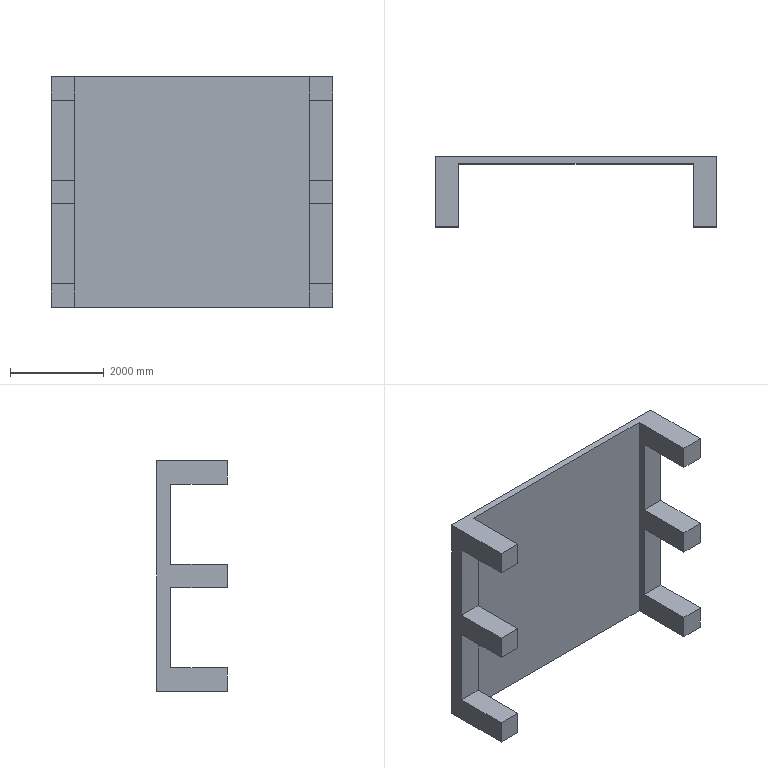Part | SolidWorks | features Extrusion 1, ICE 1 | 1 solid | 26 faces | box 6000 x 1500 x 4914 mm | volume 6959700000 mm3 | plane 26
STEP:
#1=CARTESIAN_POINT('',(2500.,-1500.,-65.));
#2=VERTEX_POINT('',#1);
#3=CARTESIAN_POINT('',(3000.,-1500.,-65.));
#4=VERTEX_POINT('',#3);
#5=CARTESIAN_POINT('',(-3000.,-1500.,-65.));
#6=DIRECTION('',(1.,0.,0.));
#7=VECTOR('',#6,1000.);
#8=LINE('',#5,#7);
#9=EDGE_CURVE('',#2,#4,#8,.T.);
#10=ORIENTED_EDGE('',*,*,#9,.T.);
#11=CARTESIAN_POINT('',(3000.,-1500.,435.));
#12=VERTEX_POINT('',#11);
#13=CARTESIAN_POINT('',(3000.,-1500.,-4479.));
#14=DIRECTION('',(0.,0.,1.));
#15=VECTOR('',#14,1000.);
#16=LINE('',#13,#15);
#17=EDGE_CURVE('',#4,#12,#16,.T.);
#18=ORIENTED_EDGE('',*,*,#17,.T.);
#19=CARTESIAN_POINT('',(2500.,-1500.,435.));
#20=VERTEX_POINT('',#19);
#21=CARTESIAN_POINT('',(3000.,-1500.,435.));
#22=DIRECTION('',(1.,0.,0.));
#23=VECTOR('',#22,1000.);
#24=LINE('',#21,#23);
#25=EDGE_CURVE('',#20,#12,#24,.T.);
#26=ORIENTED_EDGE('',*,*,#25,.F.);
#27=CARTESIAN_POINT('',(2500.,-1500.,-4479.));
#28=DIRECTION('',(0.,0.,1.));
#29=VECTOR('',#28,1000.);
#30=LINE('',#27,#29);
#31=EDGE_CURVE('',#2,#20,#30,.T.);
#32=ORIENTED_EDGE('',*,*,#31,.F.);
#33=EDGE_LOOP('',(#10,#18,#26,#32));
#34=FACE_OUTER_BOUND('',#33,.T.);
#35=CARTESIAN_POINT('',(3000.,-1500.,-4479.));
#36=DIRECTION('',(0.,-1.,0.));
#37=DIRECTION('',(1.,0.,0.));
#38=AXIS2_PLACEMENT_3D('',#35,#36,#37);
#39=PLANE('',#38);
#40=ADVANCED_FACE('',(#34),#39,.T.);
#41=CARTESIAN_POINT('',(2500.,-1500.,-1772.));
#42=VERTEX_POINT('',#41);
#43=CARTESIAN_POINT('',(3000.,-1500.,-1772.));
#44=VERTEX_POINT('',#43);
#45=CARTESIAN_POINT('',(-3000.,-1500.,-1772.));
#46=DIRECTION('',(1.,0.,0.));
#47=VECTOR('',#46,1000.);
#48=LINE('',#45,#47);
#49=EDGE_CURVE('',#42,#44,#48,.T.);
#50=ORIENTED_EDGE('',*,*,#49,.F.);
#51=CARTESIAN_POINT('',(2500.,-1500.,-2272.));
#52=VERTEX_POINT('',#51);
#53=CARTESIAN_POINT('',(2500.,-1500.,-4479.));
#54=DIRECTION('',(0.,0.,1.));
#55=VECTOR('',#54,1000.);
#56=LINE('',#53,#55);
#57=EDGE_CURVE('',#52,#42,#56,.T.);
#58=ORIENTED_EDGE('',*,*,#57,.F.);
#59=CARTESIAN_POINT('',(3000.,-1500.,-2272.));
#60=VERTEX_POINT('',#59);
#61=CARTESIAN_POINT('',(-3000.,-1500.,-2272.));
#62=DIRECTION('',(1.,0.,0.));
#63=VECTOR('',#62,1000.);
#64=LINE('',#61,#63);
#65=EDGE_CURVE('',#52,#60,#64,.T.);
#66=ORIENTED_EDGE('',*,*,#65,.T.);
#67=CARTESIAN_POINT('',(3000.,-1500.,-4479.));
#68=DIRECTION('',(0.,0.,1.));
#69=VECTOR('',#68,1000.);
#70=LINE('',#67,#69);
#71=EDGE_CURVE('',#60,#44,#70,.T.);
#72=ORIENTED_EDGE('',*,*,#71,.T.);
#73=EDGE_LOOP('',(#50,#58,#66,#72));
#74=FACE_OUTER_BOUND('',#73,.T.);
#75=CARTESIAN_POINT('',(3000.,-1500.,-4479.));
#76=DIRECTION('',(0.,-1.,0.));
#77=DIRECTION('',(1.,0.,0.));
#78=AXIS2_PLACEMENT_3D('',#75,#76,#77);
#79=PLANE('',#78);
#80=ADVANCED_FACE('',(#74),#79,.T.);
#81=CARTESIAN_POINT('',(-3000.,-1500.,-65.));
#82=VERTEX_POINT('',#81);
#83=CARTESIAN_POINT('',(-2500.,-1500.,-65.));
#84=VERTEX_POINT('',#83);
#85=CARTESIAN_POINT('',(-3000.,-1500.,-65.));
#86=DIRECTION('',(1.,0.,0.));
#87=VECTOR('',#86,1000.);
#88=LINE('',#85,#87);
#89=EDGE_CURVE('',#82,#84,#88,.T.);
#90=ORIENTED_EDGE('',*,*,#89,.T.);
#91=CARTESIAN_POINT('',(-2500.,-1500.,435.));
#92=VERTEX_POINT('',#91);
#93=CARTESIAN_POINT('',(-2500.,-1500.,-4479.));
#94=DIRECTION('',(0.,0.,1.));
#95=VECTOR('',#94,1000.);
#96=LINE('',#93,#95);
#97=EDGE_CURVE('',#84,#92,#96,.T.);
#98=ORIENTED_EDGE('',*,*,#97,.T.);
#99=CARTESIAN_POINT('',(-3000.,-1500.,435.));
#100=VERTEX_POINT('',#99);
#101=CARTESIAN_POINT('',(-2500.,-1500.,435.));
#102=DIRECTION('',(1.,0.,0.));
#103=VECTOR('',#102,1000.);
#104=LINE('',#101,#103);
#105=EDGE_CURVE('',#100,#92,#104,.T.);
#106=ORIENTED_EDGE('',*,*,#105,.F.);
#107=CARTESIAN_POINT('',(-3000.,-1500.,-4479.));
#108=DIRECTION('',(0.,0.,1.));
#109=VECTOR('',#108,1000.);
#110=LINE('',#107,#109);
#111=EDGE_CURVE('',#82,#100,#110,.T.);
#112=ORIENTED_EDGE('',*,*,#111,.F.);
#113=EDGE_LOOP('',(#90,#98,#106,#112));
#114=FACE_OUTER_BOUND('',#113,.T.);
#115=CARTESIAN_POINT('',(-2500.,-1500.,-4479.));
#116=DIRECTION('',(0.,-1.,0.));
#117=DIRECTION('',(1.,0.,0.));
#118=AXIS2_PLACEMENT_3D('',#115,#116,#117);
#119=PLANE('',#118);
#120=ADVANCED_FACE('',(#114),#119,.T.);
#121=CARTESIAN_POINT('',(-3000.,-1500.,-1772.));
#122=VERTEX_POINT('',#121);
#123=CARTESIAN_POINT('',(-2500.,-1500.,-1772.));
#124=VERTEX_POINT('',#123);
#125=CARTESIAN_POINT('',(-3000.,-1500.,-1772.));
#126=DIRECTION('',(1.,0.,0.));
#127=VECTOR('',#126,1000.);
#128=LINE('',#125,#127);
#129=EDGE_CURVE('',#122,#124,#128,.T.);
#130=ORIENTED_EDGE('',*,*,#129,.F.);
#131=CARTESIAN_POINT('',(-3000.,-1500.,-2272.));
#132=VERTEX_POINT('',#131);
#133=CARTESIAN_POINT('',(-3000.,-1500.,-4479.));
#134=DIRECTION('',(0.,0.,1.));
#135=VECTOR('',#134,1000.);
#136=LINE('',#133,#135);
#137=EDGE_CURVE('',#132,#122,#136,.T.);
#138=ORIENTED_EDGE('',*,*,#137,.F.);
#139=CARTESIAN_POINT('',(-2500.,-1500.,-2272.));
#140=VERTEX_POINT('',#139);
#141=CARTESIAN_POINT('',(-3000.,-1500.,-2272.));
#142=DIRECTION('',(1.,0.,0.));
#143=VECTOR('',#142,1000.);
#144=LINE('',#141,#143);
#145=EDGE_CURVE('',#132,#140,#144,.T.);
#146=ORIENTED_EDGE('',*,*,#145,.T.);
#147=CARTESIAN_POINT('',(-2500.,-1500.,-4479.));
#148=DIRECTION('',(0.,0.,1.));
#149=VECTOR('',#148,1000.);
#150=LINE('',#147,#149);
#151=EDGE_CURVE('',#140,#124,#150,.T.);
#152=ORIENTED_EDGE('',*,*,#151,.T.);
#153=EDGE_LOOP('',(#130,#138,#146,#152));
#154=FACE_OUTER_BOUND('',#153,.T.);
#155=CARTESIAN_POINT('',(-2500.,-1500.,-4479.));
#156=DIRECTION('',(0.,-1.,0.));
#157=DIRECTION('',(1.,0.,0.));
#158=AXIS2_PLACEMENT_3D('',#155,#156,#157);
#159=PLANE('',#158);
#160=ADVANCED_FACE('',(#154),#159,.T.);
#161=CARTESIAN_POINT('',(-3000.,-300.,-65.));
#162=VERTEX_POINT('',#161);
#163=CARTESIAN_POINT('',(-3000.,-1500.,-65.));
#164=DIRECTION('',(0.,-1.,0.));
#165=VECTOR('',#164,1000.);
#166=LINE('',#163,#165);
#167=EDGE_CURVE('',#162,#82,#166,.T.);
#168=ORIENTED_EDGE('',*,*,#167,.T.);
#169=ORIENTED_EDGE('',*,*,#111,.T.);
#170=CARTESIAN_POINT('',(-3000.,0.,435.));
#171=VERTEX_POINT('',#170);
#172=CARTESIAN_POINT('',(-3000.,-1500.,435.));
#173=DIRECTION('',(0.,-1.,0.));
#174=VECTOR('',#173,1000.);
#175=LINE('',#172,#174);
#176=EDGE_CURVE('',#171,#100,#175,.T.);
#177=ORIENTED_EDGE('',*,*,#176,.F.);
#178=CARTESIAN_POINT('',(-3000.,0.,-4479.));
#179=VERTEX_POINT('',#178);
#180=CARTESIAN_POINT('',(-3000.,0.,-4479.));
#181=DIRECTION('',(0.,0.,1.));
#182=VECTOR('',#181,1000.);
#183=LINE('',#180,#182);
#184=EDGE_CURVE('',#179,#171,#183,.T.);
#185=ORIENTED_EDGE('',*,*,#184,.F.);
#186=CARTESIAN_POINT('',(-3000.,-1500.,-4479.));
#187=VERTEX_POINT('',#186);
#188=CARTESIAN_POINT('',(-3000.,-1500.,-4479.));
#189=DIRECTION('',(0.,-1.,0.));
#190=VECTOR('',#189,1000.);
#191=LINE('',#188,#190);
#192=EDGE_CURVE('',#179,#187,#191,.T.);
#193=ORIENTED_EDGE('',*,*,#192,.T.);
#194=CARTESIAN_POINT('',(-3000.,-1500.,-3979.));
#195=VERTEX_POINT('',#194);
#196=CARTESIAN_POINT('',(-3000.,-1500.,-4479.));
#197=DIRECTION('',(0.,0.,1.));
#198=VECTOR('',#197,1000.);
#199=LINE('',#196,#198);
#200=EDGE_CURVE('',#187,#195,#199,.T.);
#201=ORIENTED_EDGE('',*,*,#200,.T.);
#202=CARTESIAN_POINT('',(-3000.,-300.,-3979.));
#203=VERTEX_POINT('',#202);
#204=CARTESIAN_POINT('',(-3000.,-1500.,-3979.));
#205=DIRECTION('',(0.,1.,0.));
#206=VECTOR('',#205,1000.);
#207=LINE('',#204,#206);
#208=EDGE_CURVE('',#195,#203,#207,.T.);
#209=ORIENTED_EDGE('',*,*,#208,.T.);
#210=CARTESIAN_POINT('',(-3000.,-300.,-2272.));
#211=VERTEX_POINT('',#210);
#212=CARTESIAN_POINT('',(-3000.,-300.,-3979.));
#213=DIRECTION('',(0.,0.,1.));
#214=VECTOR('',#213,1000.);
#215=LINE('',#212,#214);
#216=EDGE_CURVE('',#203,#211,#215,.T.);
#217=ORIENTED_EDGE('',*,*,#216,.T.);
#218=CARTESIAN_POINT('',(-3000.,-1500.,-2272.));
#219=DIRECTION('',(0.,-1.,0.));
#220=VECTOR('',#219,1000.);
#221=LINE('',#218,#220);
#222=EDGE_CURVE('',#211,#132,#221,.T.);
#223=ORIENTED_EDGE('',*,*,#222,.T.);
#224=ORIENTED_EDGE('',*,*,#137,.T.);
#225=CARTESIAN_POINT('',(-3000.,-300.,-1772.));
#226=VERTEX_POINT('',#225);
#227=CARTESIAN_POINT('',(-3000.,-1500.,-1772.));
#228=DIRECTION('',(0.,1.,0.));
#229=VECTOR('',#228,1000.);
#230=LINE('',#227,#229);
#231=EDGE_CURVE('',#122,#226,#230,.T.);
#232=ORIENTED_EDGE('',*,*,#231,.T.);
#233=CARTESIAN_POINT('',(-3000.,-300.,-65.));
#234=DIRECTION('',(0.,0.,1.));
#235=VECTOR('',#234,1000.);
#236=LINE('',#233,#235);
#237=EDGE_CURVE('',#226,#162,#236,.T.);
#238=ORIENTED_EDGE('',*,*,#237,.T.);
#239=EDGE_LOOP('',(#168,#169,#177,#185,#193,#201,#209,#217,#223,#224,#232,#238));
#240=FACE_OUTER_BOUND('',#239,.T.);
#241=CARTESIAN_POINT('',(-3000.,-1500.,-4479.));
#242=DIRECTION('',(-1.,0.,0.));
#243=DIRECTION('',(0.,0.,1.));
#244=AXIS2_PLACEMENT_3D('',#241,#242,#243);
#245=PLANE('',#244);
#246=ADVANCED_FACE('',(#240),#245,.T.);
#247=ORIENTED_EDGE('',*,*,#184,.T.);
#248=CARTESIAN_POINT('',(3000.,0.,435.));
#249=VERTEX_POINT('',#248);
#250=CARTESIAN_POINT('',(3000.,0.,435.));
#251=DIRECTION('',(-1.,0.,0.));
#252=VECTOR('',#251,1000.);
#253=LINE('',#250,#252);
#254=EDGE_CURVE('',#249,#171,#253,.T.);
#255=ORIENTED_EDGE('',*,*,#254,.F.);
#256=CARTESIAN_POINT('',(3000.,0.,-4479.));
#257=VERTEX_POINT('',#256);
#258=CARTESIAN_POINT('',(3000.,0.,-4479.));
#259=DIRECTION('',(0.,0.,1.));
#260=VECTOR('',#259,1000.);
#261=LINE('',#258,#260);
#262=EDGE_CURVE('',#257,#249,#261,.T.);
#263=ORIENTED_EDGE('',*,*,#262,.F.);
#264=CARTESIAN_POINT('',(3000.,0.,-4479.));
#265=DIRECTION('',(-1.,0.,0.));
#266=VECTOR('',#265,1000.);
#267=LINE('',#264,#266);
#268=EDGE_CURVE('',#257,#179,#267,.T.);
#269=ORIENTED_EDGE('',*,*,#268,.T.);
#270=EDGE_LOOP('',(#247,#255,#263,#269));
#271=FACE_OUTER_BOUND('',#270,.T.);
#272=CARTESIAN_POINT('',(3000.,0.,-4479.));
#273=DIRECTION('',(0.,1.,0.));
#274=DIRECTION('',(-1.,0.,0.));
#275=AXIS2_PLACEMENT_3D('',#272,#273,#274);
#276=PLANE('',#275);
#277=ADVANCED_FACE('',(#271),#276,.T.);
#278=CARTESIAN_POINT('',(3000.,-300.,-65.));
#279=VERTEX_POINT('',#278);
#280=CARTESIAN_POINT('',(3000.,-1500.,-65.));
#281=DIRECTION('',(0.,-1.,0.));
#282=VECTOR('',#281,1000.);
#283=LINE('',#280,#282);
#284=EDGE_CURVE('',#279,#4,#283,.T.);
#285=ORIENTED_EDGE('',*,*,#284,.F.);
#286=CARTESIAN_POINT('',(3000.,-300.,-1772.));
#287=VERTEX_POINT('',#286);
#288=CARTESIAN_POINT('',(3000.,-300.,-65.));
#289=DIRECTION('',(0.,0.,1.));
#290=VECTOR('',#289,1000.);
#291=LINE('',#288,#290);
#292=EDGE_CURVE('',#287,#279,#291,.T.);
#293=ORIENTED_EDGE('',*,*,#292,.F.);
#294=CARTESIAN_POINT('',(3000.,-1500.,-1772.));
#295=DIRECTION('',(0.,1.,0.));
#296=VECTOR('',#295,1000.);
#297=LINE('',#294,#296);
#298=EDGE_CURVE('',#44,#287,#297,.T.);
#299=ORIENTED_EDGE('',*,*,#298,.F.);
#300=ORIENTED_EDGE('',*,*,#71,.F.);
#301=CARTESIAN_POINT('',(3000.,-300.,-2272.));
#302=VERTEX_POINT('',#301);
#303=CARTESIAN_POINT('',(3000.,-1500.,-2272.));
#304=DIRECTION('',(0.,-1.,0.));
#305=VECTOR('',#304,1000.);
#306=LINE('',#303,#305);
#307=EDGE_CURVE('',#302,#60,#306,.T.);
#308=ORIENTED_EDGE('',*,*,#307,.F.);
#309=CARTESIAN_POINT('',(3000.,-300.,-3979.));
#310=VERTEX_POINT('',#309);
#311=CARTESIAN_POINT('',(3000.,-300.,-3979.));
#312=DIRECTION('',(0.,0.,1.));
#313=VECTOR('',#312,1000.);
#314=LINE('',#311,#313);
#315=EDGE_CURVE('',#310,#302,#314,.T.);
#316=ORIENTED_EDGE('',*,*,#315,.F.);
#317=CARTESIAN_POINT('',(3000.,-1500.,-3979.));
#318=VERTEX_POINT('',#317);
#319=CARTESIAN_POINT('',(3000.,-1500.,-3979.));
#320=DIRECTION('',(0.,1.,0.));
#321=VECTOR('',#320,1000.);
#322=LINE('',#319,#321);
#323=EDGE_CURVE('',#318,#310,#322,.T.);
#324=ORIENTED_EDGE('',*,*,#323,.F.);
#325=CARTESIAN_POINT('',(3000.,-1500.,-4479.));
#326=VERTEX_POINT('',#325);
#327=CARTESIAN_POINT('',(3000.,-1500.,-4479.));
#328=DIRECTION('',(0.,0.,1.));
#329=VECTOR('',#328,1000.);
#330=LINE('',#327,#329);
#331=EDGE_CURVE('',#326,#318,#330,.T.);
#332=ORIENTED_EDGE('',*,*,#331,.F.);
#333=CARTESIAN_POINT('',(3000.,-1500.,-4479.));
#334=DIRECTION('',(0.,1.,0.));
#335=VECTOR('',#334,1000.);
#336=LINE('',#333,#335);
#337=EDGE_CURVE('',#326,#257,#336,.T.);
#338=ORIENTED_EDGE('',*,*,#337,.T.);
#339=ORIENTED_EDGE('',*,*,#262,.T.);
#340=CARTESIAN_POINT('',(3000.,-1500.,435.));
#341=DIRECTION('',(0.,1.,0.));
#342=VECTOR('',#341,1000.);
#343=LINE('',#340,#342);
#344=EDGE_CURVE('',#12,#249,#343,.T.);
#345=ORIENTED_EDGE('',*,*,#344,.F.);
#346=ORIENTED_EDGE('',*,*,#17,.F.);
#347=EDGE_LOOP('',(#285,#293,#299,#300,#308,#316,#324,#332,#338,#339,#345,#346));
#348=FACE_OUTER_BOUND('',#347,.T.);
#349=CARTESIAN_POINT('',(3000.,-1500.,-4479.));
#350=DIRECTION('',(1.,0.,0.));
#351=DIRECTION('',(0.,0.,-1.));
#352=AXIS2_PLACEMENT_3D('',#349,#350,#351);
#353=PLANE('',#352);
#354=ADVANCED_FACE('',(#348),#353,.T.);
#355=CARTESIAN_POINT('',(2500.,-1500.,-3979.));
#356=VERTEX_POINT('',#355);
#357=CARTESIAN_POINT('',(-3000.,-1500.,-3979.));
#358=DIRECTION('',(1.,0.,0.));
#359=VECTOR('',#358,1000.);
#360=LINE('',#357,#359);
#361=EDGE_CURVE('',#356,#318,#360,.T.);
#362=ORIENTED_EDGE('',*,*,#361,.F.);
#363=CARTESIAN_POINT('',(2500.,-1500.,-4479.));
#364=VERTEX_POINT('',#363);
#365=CARTESIAN_POINT('',(2500.,-1500.,-4479.));
#366=DIRECTION('',(0.,0.,1.));
#367=VECTOR('',#366,1000.);
#368=LINE('',#365,#367);
#369=EDGE_CURVE('',#364,#356,#368,.T.);
#370=ORIENTED_EDGE('',*,*,#369,.F.);
#371=CARTESIAN_POINT('',(3000.,-1500.,-4479.));
#372=DIRECTION('',(1.,0.,0.));
#373=VECTOR('',#372,1000.);
#374=LINE('',#371,#373);
#375=EDGE_CURVE('',#364,#326,#374,.T.);
#376=ORIENTED_EDGE('',*,*,#375,.T.);
#377=ORIENTED_EDGE('',*,*,#331,.T.);
#378=EDGE_LOOP('',(#362,#370,#376,#377));
#379=FACE_OUTER_BOUND('',#378,.T.);
#380=CARTESIAN_POINT('',(3000.,-1500.,-4479.));
#381=DIRECTION('',(0.,-1.,0.));
#382=DIRECTION('',(1.,0.,0.));
#383=AXIS2_PLACEMENT_3D('',#380,#381,#382);
#384=PLANE('',#383);
#385=ADVANCED_FACE('',(#379),#384,.T.);
#386=CARTESIAN_POINT('',(2500.,-300.,-65.));
#387=VERTEX_POINT('',#386);
#388=CARTESIAN_POINT('',(2500.,-1500.,-65.));
#389=DIRECTION('',(0.,1.,0.));
#390=VECTOR('',#389,1000.);
#391=LINE('',#388,#390);
#392=EDGE_CURVE('',#2,#387,#391,.T.);
#393=ORIENTED_EDGE('',*,*,#392,.F.);
#394=ORIENTED_EDGE('',*,*,#31,.T.);
#395=CARTESIAN_POINT('',(2500.,-150.,435.));
#396=VERTEX_POINT('',#395);
#397=CARTESIAN_POINT('',(2500.,-1500.,435.));
#398=DIRECTION('',(0.,-1.,0.));
#399=VECTOR('',#398,1000.);
#400=LINE('',#397,#399);
#401=EDGE_CURVE('',#396,#20,#400,.T.);
#402=ORIENTED_EDGE('',*,*,#401,.F.);
#403=CARTESIAN_POINT('',(2500.,-150.,-4479.));
#404=VERTEX_POINT('',#403);
#405=CARTESIAN_POINT('',(2500.,-150.,-4479.));
#406=DIRECTION('',(0.,0.,1.));
#407=VECTOR('',#406,1000.);
#408=LINE('',#405,#407);
#409=EDGE_CURVE('',#404,#396,#408,.T.);
#410=ORIENTED_EDGE('',*,*,#409,.F.);
#411=CARTESIAN_POINT('',(2500.,-1500.,-4479.));
#412=DIRECTION('',(0.,-1.,0.));
#413=VECTOR('',#412,1000.);
#414=LINE('',#411,#413);
#415=EDGE_CURVE('',#404,#364,#414,.T.);
#416=ORIENTED_EDGE('',*,*,#415,.T.);
#417=ORIENTED_EDGE('',*,*,#369,.T.);
#418=CARTESIAN_POINT('',(2500.,-300.,-3979.));
#419=VERTEX_POINT('',#418);
#420=CARTESIAN_POINT('',(2500.,-1500.,-3979.));
#421=DIRECTION('',(0.,-1.,0.));
#422=VECTOR('',#421,1000.);
#423=LINE('',#420,#422);
#424=EDGE_CURVE('',#419,#356,#423,.T.);
#425=ORIENTED_EDGE('',*,*,#424,.F.);
#426=CARTESIAN_POINT('',(2500.,-300.,-2272.));
#427=VERTEX_POINT('',#426);
#428=CARTESIAN_POINT('',(2500.,-300.,-4479.));
#429=DIRECTION('',(0.,0.,-1.));
#430=VECTOR('',#429,1000.);
#431=LINE('',#428,#430);
#432=EDGE_CURVE('',#427,#419,#431,.T.);
#433=ORIENTED_EDGE('',*,*,#432,.F.);
#434=CARTESIAN_POINT('',(2500.,-1500.,-2272.));
#435=DIRECTION('',(0.,1.,0.));
#436=VECTOR('',#435,1000.);
#437=LINE('',#434,#436);
#438=EDGE_CURVE('',#52,#427,#437,.T.);
#439=ORIENTED_EDGE('',*,*,#438,.F.);
#440=ORIENTED_EDGE('',*,*,#57,.T.);
#441=CARTESIAN_POINT('',(2500.,-300.,-1772.));
#442=VERTEX_POINT('',#441);
#443=CARTESIAN_POINT('',(2500.,-1500.,-1772.));
#444=DIRECTION('',(0.,-1.,0.));
#445=VECTOR('',#444,1000.);
#446=LINE('',#443,#445);
#447=EDGE_CURVE('',#442,#42,#446,.T.);
#448=ORIENTED_EDGE('',*,*,#447,.F.);
#449=CARTESIAN_POINT('',(2500.,-300.,-4479.));
#450=DIRECTION('',(0.,0.,-1.));
#451=VECTOR('',#450,1000.);
#452=LINE('',#449,#451);
#453=EDGE_CURVE('',#387,#442,#452,.T.);
#454=ORIENTED_EDGE('',*,*,#453,.F.);
#455=EDGE_LOOP('',(#393,#394,#402,#410,#416,#417,#425,#433,#439,#440,#448,#454));
#456=FACE_OUTER_BOUND('',#455,.T.);
#457=CARTESIAN_POINT('',(2500.,-1500.,-4479.));
#458=DIRECTION('',(-1.,0.,0.));
#459=DIRECTION('',(0.,-1.,0.));
#460=AXIS2_PLACEMENT_3D('',#457,#458,#459);
#461=PLANE('',#460);
#462=ADVANCED_FACE('',(#456),#461,.T.);
#463=ORIENTED_EDGE('',*,*,#409,.T.);
#464=CARTESIAN_POINT('',(-2500.,-150.,435.));
#465=VERTEX_POINT('',#464);
#466=CARTESIAN_POINT('',(-2500.,-150.,435.));
#467=DIRECTION('',(1.,0.,0.));
#468=VECTOR('',#467,1000.);
#469=LINE('',#466,#468);
#470=EDGE_CURVE('',#465,#396,#469,.T.);
#471=ORIENTED_EDGE('',*,*,#470,.F.);
#472=CARTESIAN_POINT('',(-2500.,-150.,-4479.));
#473=VERTEX_POINT('',#472);
#474=CARTESIAN_POINT('',(-2500.,-150.,-4479.));
#475=DIRECTION('',(0.,0.,1.));
#476=VECTOR('',#475,1000.);
#477=LINE('',#474,#476);
#478=EDGE_CURVE('',#473,#465,#477,.T.);
#479=ORIENTED_EDGE('',*,*,#478,.F.);
#480=CARTESIAN_POINT('',(-2500.,-150.,-4479.));
#481=DIRECTION('',(1.,0.,0.));
#482=VECTOR('',#481,1000.);
#483=LINE('',#480,#482);
#484=EDGE_CURVE('',#473,#404,#483,.T.);
#485=ORIENTED_EDGE('',*,*,#484,.T.);
#486=EDGE_LOOP('',(#463,#471,#479,#485));
#487=FACE_OUTER_BOUND('',#486,.T.);
#488=CARTESIAN_POINT('',(-2500.,-150.,-4479.));
#489=DIRECTION('',(0.,-1.,0.));
#490=DIRECTION('',(1.,0.,0.));
#491=AXIS2_PLACEMENT_3D('',#488,#489,#490);
#492=PLANE('',#491);
#493=ADVANCED_FACE('',(#487),#492,.T.);
#494=CARTESIAN_POINT('',(-2500.,-300.,-65.));
#495=VERTEX_POINT('',#494);
#496=CARTESIAN_POINT('',(-2500.,-1500.,-65.));
#497=DIRECTION('',(0.,-1.,0.));
#498=VECTOR('',#497,1000.);
#499=LINE('',#496,#498);
#500=EDGE_CURVE('',#495,#84,#499,.T.);
#501=ORIENTED_EDGE('',*,*,#500,.F.);
#502=CARTESIAN_POINT('',(-2500.,-300.,-1772.));
#503=VERTEX_POINT('',#502);
#504=CARTESIAN_POINT('',(-2500.,-300.,-4479.));
#505=DIRECTION('',(0.,0.,1.));
#506=VECTOR('',#505,1000.);
#507=LINE('',#504,#506);
#508=EDGE_CURVE('',#503,#495,#507,.T.);
#509=ORIENTED_EDGE('',*,*,#508,.F.);
#510=CARTESIAN_POINT('',(-2500.,-1500.,-1772.));
#511=DIRECTION('',(0.,1.,0.));
#512=VECTOR('',#511,1000.);
#513=LINE('',#510,#512);
#514=EDGE_CURVE('',#124,#503,#513,.T.);
#515=ORIENTED_EDGE('',*,*,#514,.F.);
#516=ORIENTED_EDGE('',*,*,#151,.F.);
#517=CARTESIAN_POINT('',(-2500.,-300.,-2272.));
#518=VERTEX_POINT('',#517);
#519=CARTESIAN_POINT('',(-2500.,-1500.,-2272.));
#520=DIRECTION('',(0.,-1.,0.));
#521=VECTOR('',#520,1000.);
#522=LINE('',#519,#521);
#523=EDGE_CURVE('',#518,#140,#522,.T.);
#524=ORIENTED_EDGE('',*,*,#523,.F.);
#525=CARTESIAN_POINT('',(-2500.,-300.,-3979.));
#526=VERTEX_POINT('',#525);
#527=CARTESIAN_POINT('',(-2500.,-300.,-4479.));
#528=DIRECTION('',(0.,0.,1.));
#529=VECTOR('',#528,1000.);
#530=LINE('',#527,#529);
#531=EDGE_CURVE('',#526,#518,#530,.T.);
#532=ORIENTED_EDGE('',*,*,#531,.F.);
#533=CARTESIAN_POINT('',(-2500.,-1500.,-3979.));
#534=VERTEX_POINT('',#533);
#535=CARTESIAN_POINT('',(-2500.,-1500.,-3979.));
#536=DIRECTION('',(0.,1.,0.));
#537=VECTOR('',#536,1000.);
#538=LINE('',#535,#537);
#539=EDGE_CURVE('',#534,#526,#538,.T.);
#540=ORIENTED_EDGE('',*,*,#539,.F.);
#541=CARTESIAN_POINT('',(-2500.,-1500.,-4479.));
#542=VERTEX_POINT('',#541);
#543=CARTESIAN_POINT('',(-2500.,-1500.,-4479.));
#544=DIRECTION('',(0.,0.,1.));
#545=VECTOR('',#544,1000.);
#546=LINE('',#543,#545);
#547=EDGE_CURVE('',#542,#534,#546,.T.);
#548=ORIENTED_EDGE('',*,*,#547,.F.);
#549=CARTESIAN_POINT('',(-2500.,-1500.,-4479.));
#550=DIRECTION('',(0.,1.,0.));
#551=VECTOR('',#550,1000.);
#552=LINE('',#549,#551);
#553=EDGE_CURVE('',#542,#473,#552,.T.);
#554=ORIENTED_EDGE('',*,*,#553,.T.);
#555=ORIENTED_EDGE('',*,*,#478,.T.);
#556=CARTESIAN_POINT('',(-2500.,-1500.,435.));
#557=DIRECTION('',(0.,1.,0.));
#558=VECTOR('',#557,1000.);
#559=LINE('',#556,#558);
#560=EDGE_CURVE('',#92,#465,#559,.T.);
#561=ORIENTED_EDGE('',*,*,#560,.F.);
#562=ORIENTED_EDGE('',*,*,#97,.F.);
#563=EDGE_LOOP('',(#501,#509,#515,#516,#524,#532,#540,#548,#554,#555,#561,#562));
#564=FACE_OUTER_BOUND('',#563,.T.);
#565=CARTESIAN_POINT('',(-2500.,-1500.,-4479.));
#566=DIRECTION('',(1.,0.,0.));
#567=DIRECTION('',(0.,1.,0.));
#568=AXIS2_PLACEMENT_3D('',#565,#566,#567);
#569=PLANE('',#568);
#570=ADVANCED_FACE('',(#564),#569,.T.);
#571=CARTESIAN_POINT('',(-3000.,-1500.,-3979.));
#572=DIRECTION('',(1.,0.,0.));
#573=VECTOR('',#572,1000.);
#574=LINE('',#571,#573);
#575=EDGE_CURVE('',#195,#534,#574,.T.);
#576=ORIENTED_EDGE('',*,*,#575,.F.);
#577=ORIENTED_EDGE('',*,*,#200,.F.);
#578=CARTESIAN_POINT('',(-2500.,-1500.,-4479.));
#579=DIRECTION('',(1.,0.,0.));
#580=VECTOR('',#579,1000.);
#581=LINE('',#578,#580);
#582=EDGE_CURVE('',#187,#542,#581,.T.);
#583=ORIENTED_EDGE('',*,*,#582,.T.);
#584=ORIENTED_EDGE('',*,*,#547,.T.);
#585=EDGE_LOOP('',(#576,#577,#583,#584));
#586=FACE_OUTER_BOUND('',#585,.T.);
#587=CARTESIAN_POINT('',(-2500.,-1500.,-4479.));
#588=DIRECTION('',(0.,-1.,0.));
#589=DIRECTION('',(1.,0.,0.));
#590=AXIS2_PLACEMENT_3D('',#587,#588,#589);
#591=PLANE('',#590);
#592=ADVANCED_FACE('',(#586),#591,.T.);
#593=ORIENTED_EDGE('',*,*,#192,.F.);
#594=ORIENTED_EDGE('',*,*,#268,.F.);
#595=ORIENTED_EDGE('',*,*,#337,.F.);
#596=ORIENTED_EDGE('',*,*,#375,.F.);
#597=ORIENTED_EDGE('',*,*,#415,.F.);
#598=ORIENTED_EDGE('',*,*,#484,.F.);
#599=ORIENTED_EDGE('',*,*,#553,.F.);
#600=ORIENTED_EDGE('',*,*,#582,.F.);
#601=EDGE_LOOP('',(#593,#594,#595,#596,#597,#598,#599,#600));
#602=FACE_OUTER_BOUND('',#601,.T.);
#603=CARTESIAN_POINT('',(0.,0.,-4479.));
#604=DIRECTION('',(0.,0.,1.));
#605=DIRECTION('',(1.,0.,0.));
#606=AXIS2_PLACEMENT_3D('',#603,#604,#605);
#607=PLANE('',#606);
#608=ADVANCED_FACE('',(#602),#607,.F.);
#609=ORIENTED_EDGE('',*,*,#176,.T.);
#610=ORIENTED_EDGE('',*,*,#105,.T.);
#611=ORIENTED_EDGE('',*,*,#560,.T.);
#612=ORIENTED_EDGE('',*,*,#470,.T.);
#613=ORIENTED_EDGE('',*,*,#401,.T.);
#614=ORIENTED_EDGE('',*,*,#25,.T.);
#615=ORIENTED_EDGE('',*,*,#344,.T.);
#616=ORIENTED_EDGE('',*,*,#254,.T.);
#617=EDGE_LOOP('',(#609,#610,#611,#612,#613,#614,#615,#616));
#618=FACE_OUTER_BOUND('',#617,.T.);
#619=CARTESIAN_POINT('',(0.,0.,435.));
#620=DIRECTION('',(0.,0.,1.));
#621=DIRECTION('',(1.,0.,0.));
#622=AXIS2_PLACEMENT_3D('',#619,#620,#621);
#623=PLANE('',#622);
#624=ADVANCED_FACE('',(#618),#623,.T.);
#625=ORIENTED_EDGE('',*,*,#523,.T.);
#626=ORIENTED_EDGE('',*,*,#145,.F.);
#627=ORIENTED_EDGE('',*,*,#222,.F.);
#628=CARTESIAN_POINT('',(-3000.,-300.,-2272.));
#629=DIRECTION('',(1.,0.,0.));
#630=VECTOR('',#629,1000.);
#631=LINE('',#628,#630);
#632=EDGE_CURVE('',#211,#518,#631,.T.);
#633=ORIENTED_EDGE('',*,*,#632,.T.);
#634=EDGE_LOOP('',(#625,#626,#627,#633));
#635=FACE_OUTER_BOUND('',#634,.T.);
#636=CARTESIAN_POINT('',(-3000.,-1500.,-2272.));
#637=DIRECTION('',(0.,0.,1.));
#638=DIRECTION('',(1.,0.,0.));
#639=AXIS2_PLACEMENT_3D('',#636,#637,#638);
#640=PLANE('',#639);
#641=ADVANCED_FACE('',(#635),#640,.F.);
#642=ORIENTED_EDGE('',*,*,#539,.T.);
#643=CARTESIAN_POINT('',(-3000.,-300.,-3979.));
#644=DIRECTION('',(1.,0.,0.));
#645=VECTOR('',#644,1000.);
#646=LINE('',#643,#645);
#647=EDGE_CURVE('',#203,#526,#646,.T.);
#648=ORIENTED_EDGE('',*,*,#647,.F.);
#649=ORIENTED_EDGE('',*,*,#208,.F.);
#650=ORIENTED_EDGE('',*,*,#575,.T.);
#651=EDGE_LOOP('',(#642,#648,#649,#650));
#652=FACE_OUTER_BOUND('',#651,.T.);
#653=CARTESIAN_POINT('',(-3000.,-1500.,-3979.));
#654=DIRECTION('',(0.,0.,-1.));
#655=DIRECTION('',(-1.,0.,0.));
#656=AXIS2_PLACEMENT_3D('',#653,#654,#655);
#657=PLANE('',#656);
#658=ADVANCED_FACE('',(#652),#657,.F.);
#659=ORIENTED_EDGE('',*,*,#531,.T.);
#660=ORIENTED_EDGE('',*,*,#632,.F.);
#661=ORIENTED_EDGE('',*,*,#216,.F.);
#662=ORIENTED_EDGE('',*,*,#647,.T.);
#663=EDGE_LOOP('',(#659,#660,#661,#662));
#664=FACE_OUTER_BOUND('',#663,.T.);
#665=CARTESIAN_POINT('',(-3000.,-300.,-3979.));
#666=DIRECTION('',(0.,1.,0.));
#667=DIRECTION('',(0.,0.,1.));
#668=AXIS2_PLACEMENT_3D('',#665,#666,#667);
#669=PLANE('',#668);
#670=ADVANCED_FACE('',(#664),#669,.F.);
#671=ORIENTED_EDGE('',*,*,#500,.T.);
#672=ORIENTED_EDGE('',*,*,#89,.F.);
#673=ORIENTED_EDGE('',*,*,#167,.F.);
#674=CARTESIAN_POINT('',(-3000.,-300.,-65.));
#675=DIRECTION('',(1.,0.,0.));
#676=VECTOR('',#675,1000.);
#677=LINE('',#674,#676);
#678=EDGE_CURVE('',#162,#495,#677,.T.);
#679=ORIENTED_EDGE('',*,*,#678,.T.);
#680=EDGE_LOOP('',(#671,#672,#673,#679));
#681=FACE_OUTER_BOUND('',#680,.T.);
#682=CARTESIAN_POINT('',(-3000.,-1500.,-65.));
#683=DIRECTION('',(0.,0.,1.));
#684=DIRECTION('',(1.,0.,0.));
#685=AXIS2_PLACEMENT_3D('',#682,#683,#684);
#686=PLANE('',#685);
#687=ADVANCED_FACE('',(#681),#686,.F.);
#688=ORIENTED_EDGE('',*,*,#514,.T.);
#689=CARTESIAN_POINT('',(-3000.,-300.,-1772.));
#690=DIRECTION('',(1.,0.,0.));
#691=VECTOR('',#690,1000.);
#692=LINE('',#689,#691);
#693=EDGE_CURVE('',#226,#503,#692,.T.);
#694=ORIENTED_EDGE('',*,*,#693,.F.);
#695=ORIENTED_EDGE('',*,*,#231,.F.);
#696=ORIENTED_EDGE('',*,*,#129,.T.);
#697=EDGE_LOOP('',(#688,#694,#695,#696));
#698=FACE_OUTER_BOUND('',#697,.T.);
#699=CARTESIAN_POINT('',(-3000.,-1500.,-1772.));
#700=DIRECTION('',(0.,0.,-1.));
#701=DIRECTION('',(-1.,0.,0.));
#702=AXIS2_PLACEMENT_3D('',#699,#700,#701);
#703=PLANE('',#702);
#704=ADVANCED_FACE('',(#698),#703,.F.);
#705=ORIENTED_EDGE('',*,*,#508,.T.);
#706=ORIENTED_EDGE('',*,*,#678,.F.);
#707=ORIENTED_EDGE('',*,*,#237,.F.);
#708=ORIENTED_EDGE('',*,*,#693,.T.);
#709=EDGE_LOOP('',(#705,#706,#707,#708));
#710=FACE_OUTER_BOUND('',#709,.T.);
#711=CARTESIAN_POINT('',(-3000.,-300.,-65.));
#712=DIRECTION('',(0.,1.,0.));
#713=DIRECTION('',(0.,0.,1.));
#714=AXIS2_PLACEMENT_3D('',#711,#712,#713);
#715=PLANE('',#714);
#716=ADVANCED_FACE('',(#710),#715,.F.);
#717=ORIENTED_EDGE('',*,*,#432,.T.);
#718=CARTESIAN_POINT('',(-3000.,-300.,-3979.));
#719=DIRECTION('',(1.,0.,0.));
#720=VECTOR('',#719,1000.);
#721=LINE('',#718,#720);
#722=EDGE_CURVE('',#419,#310,#721,.T.);
#723=ORIENTED_EDGE('',*,*,#722,.T.);
#724=ORIENTED_EDGE('',*,*,#315,.T.);
#725=CARTESIAN_POINT('',(-3000.,-300.,-2272.));
#726=DIRECTION('',(1.,0.,0.));
#727=VECTOR('',#726,1000.);
#728=LINE('',#725,#727);
#729=EDGE_CURVE('',#427,#302,#728,.T.);
#730=ORIENTED_EDGE('',*,*,#729,.F.);
#731=EDGE_LOOP('',(#717,#723,#724,#730));
#732=FACE_OUTER_BOUND('',#731,.T.);
#733=CARTESIAN_POINT('',(-3000.,-300.,-3979.));
#734=DIRECTION('',(0.,1.,0.));
#735=DIRECTION('',(0.,0.,1.));
#736=AXIS2_PLACEMENT_3D('',#733,#734,#735);
#737=PLANE('',#736);
#738=ADVANCED_FACE('',(#732),#737,.F.);
#739=ORIENTED_EDGE('',*,*,#438,.T.);
#740=ORIENTED_EDGE('',*,*,#729,.T.);
#741=ORIENTED_EDGE('',*,*,#307,.T.);
#742=ORIENTED_EDGE('',*,*,#65,.F.);
#743=EDGE_LOOP('',(#739,#740,#741,#742));
#744=FACE_OUTER_BOUND('',#743,.T.);
#745=CARTESIAN_POINT('',(-3000.,-1500.,-2272.));
#746=DIRECTION('',(0.,0.,1.));
#747=DIRECTION('',(1.,0.,0.));
#748=AXIS2_PLACEMENT_3D('',#745,#746,#747);
#749=PLANE('',#748);
#750=ADVANCED_FACE('',(#744),#749,.F.);
#751=ORIENTED_EDGE('',*,*,#424,.T.);
#752=ORIENTED_EDGE('',*,*,#361,.T.);
#753=ORIENTED_EDGE('',*,*,#323,.T.);
#754=ORIENTED_EDGE('',*,*,#722,.F.);
#755=EDGE_LOOP('',(#751,#752,#753,#754));
#756=FACE_OUTER_BOUND('',#755,.T.);
#757=CARTESIAN_POINT('',(-3000.,-1500.,-3979.));
#758=DIRECTION('',(0.,0.,-1.));
#759=DIRECTION('',(-1.,0.,0.));
#760=AXIS2_PLACEMENT_3D('',#757,#758,#759);
#761=PLANE('',#760);
#762=ADVANCED_FACE('',(#756),#761,.F.);
#763=ORIENTED_EDGE('',*,*,#453,.T.);
#764=CARTESIAN_POINT('',(-3000.,-300.,-1772.));
#765=DIRECTION('',(1.,0.,0.));
#766=VECTOR('',#765,1000.);
#767=LINE('',#764,#766);
#768=EDGE_CURVE('',#442,#287,#767,.T.);
#769=ORIENTED_EDGE('',*,*,#768,.T.);
#770=ORIENTED_EDGE('',*,*,#292,.T.);
#771=CARTESIAN_POINT('',(-3000.,-300.,-65.));
#772=DIRECTION('',(1.,0.,0.));
#773=VECTOR('',#772,1000.);
#774=LINE('',#771,#773);
#775=EDGE_CURVE('',#387,#279,#774,.T.);
#776=ORIENTED_EDGE('',*,*,#775,.F.);
#777=EDGE_LOOP('',(#763,#769,#770,#776));
#778=FACE_OUTER_BOUND('',#777,.T.);
#779=CARTESIAN_POINT('',(-3000.,-300.,-65.));
#780=DIRECTION('',(0.,1.,0.));
#781=DIRECTION('',(0.,0.,1.));
#782=AXIS2_PLACEMENT_3D('',#779,#780,#781);
#783=PLANE('',#782);
#784=ADVANCED_FACE('',(#778),#783,.F.);
#785=ORIENTED_EDGE('',*,*,#392,.T.);
#786=ORIENTED_EDGE('',*,*,#775,.T.);
#787=ORIENTED_EDGE('',*,*,#284,.T.);
#788=ORIENTED_EDGE('',*,*,#9,.F.);
#789=EDGE_LOOP('',(#785,#786,#787,#788));
#790=FACE_OUTER_BOUND('',#789,.T.);
#791=CARTESIAN_POINT('',(-3000.,-1500.,-65.));
#792=DIRECTION('',(0.,0.,1.));
#793=DIRECTION('',(1.,0.,0.));
#794=AXIS2_PLACEMENT_3D('',#791,#792,#793);
#795=PLANE('',#794);
#796=ADVANCED_FACE('',(#790),#795,.F.);
#797=ORIENTED_EDGE('',*,*,#447,.T.);
#798=ORIENTED_EDGE('',*,*,#49,.T.);
#799=ORIENTED_EDGE('',*,*,#298,.T.);
#800=ORIENTED_EDGE('',*,*,#768,.F.);
#801=EDGE_LOOP('',(#797,#798,#799,#800));
#802=FACE_OUTER_BOUND('',#801,.T.);
#803=CARTESIAN_POINT('',(-3000.,-1500.,-1772.));
#804=DIRECTION('',(0.,0.,-1.));
#805=DIRECTION('',(-1.,0.,0.));
#806=AXIS2_PLACEMENT_3D('',#803,#804,#805);
#807=PLANE('',#806);
#808=ADVANCED_FACE('',(#802),#807,.F.);
#809=CLOSED_SHELL('',(#40,#80,#120,#160,#246,#277,#354,#385,#462,#493,#570,#592,#608,#624,#641,#658,#670,#687,#704,#716,#738,#750,#762,#784,#796,#808));
#810=MANIFOLD_SOLID_BREP('',#809);
#811=CARTESIAN_POINT('',(0.,0.,0.));
#812=DIRECTION('',(0.,0.,1.));
#813=DIRECTION('',(1.,0.,0.));
#814=AXIS2_PLACEMENT_3D('',#811,#812,#813);
#815=(LENGTH_UNIT()NAMED_UNIT(*)SI_UNIT(.MILLI.,.METRE.));
#816=UNCERTAINTY_MEASURE_WITH_UNIT(LENGTH_MEASURE(0.00001),#815,'','');
#817=(NAMED_UNIT(*)PLANE_ANGLE_UNIT()SI_UNIT($,.RADIAN.));
#818=(NAMED_UNIT(*)SI_UNIT($,.STERADIAN.)SOLID_ANGLE_UNIT());
#819=(GEOMETRIC_REPRESENTATION_CONTEXT(3)GLOBAL_UNCERTAINTY_ASSIGNED_CONTEXT((#816))GLOBAL_UNIT_ASSIGNED_CONTEXT((#815,#817,#818))REPRESENTATION_CONTEXT('',''));
#820=ADVANCED_BREP_SHAPE_REPRESENTATION('',(#810,#814),#819);